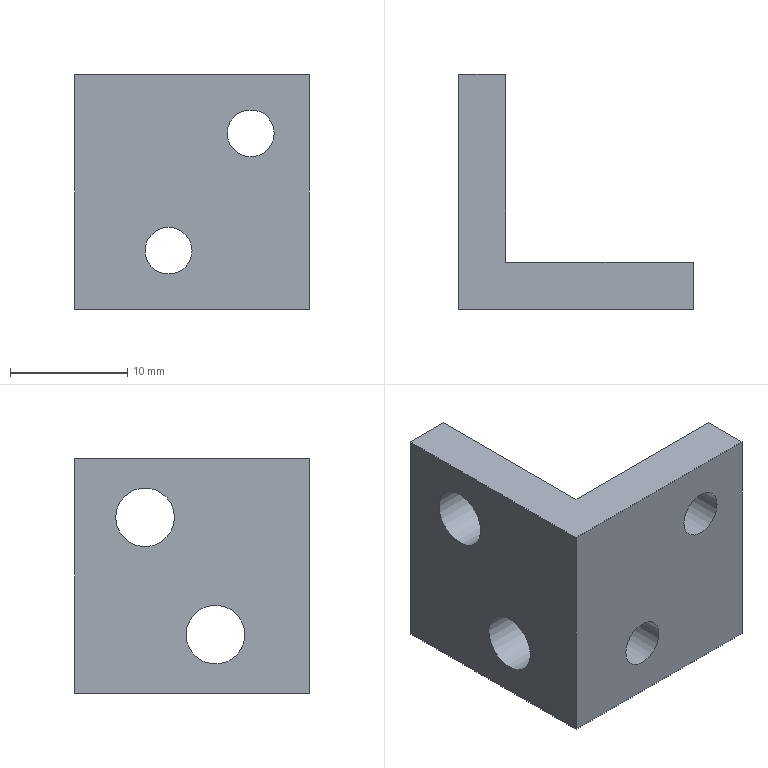Part | STEP file | 1-40.4 | 1 solid | 12 faces | box 20 x 20 x 20 mm | volume 2622 mm3 | plane 8 | cylinder 4 | commonest cylinder face diameters 4 x2 5 x2
STEP:
#1=CARTESIAN_POINT('',(0.,0.,0.));
#2=DIRECTION('',(0.,0.,1.));
#3=DIRECTION('',(1.,0.,0.));
#4=AXIS2_PLACEMENT_3D('',#1,#2,#3);
#5=CARTESIAN_POINT('',(-4.,-10.,-10.));
#6=VERTEX_POINT('',#5);
#7=CARTESIAN_POINT('',(-4.,10.,-10.));
#8=VERTEX_POINT('',#7);
#9=CARTESIAN_POINT('',(-4.,-10.,-10.));
#10=DIRECTION('',(0.,1.,0.));
#11=VECTOR('',#10,1.);
#12=LINE('',#9,#11);
#13=CARTESIAN_POINT('',(-4.,0.,0.));
#14=DIRECTION('',(1.,0.,0.));
#15=DIRECTION('',(0.,1.,0.));
#16=AXIS2_PLACEMENT_3D('',#13,#14,#15);
#17=PLANE('',#16);
#18=CARTESIAN_POINT('',(-10.,-10.));
#19=DIRECTION('',(1.,0.));
#20=VECTOR('',#19,1.);
#21=LINE('',#18,#20);
#22=(GEOMETRIC_REPRESENTATION_CONTEXT(2)PARAMETRIC_REPRESENTATION_CONTEXT()REPRESENTATION_CONTEXT('',''));
#23=DEFINITIONAL_REPRESENTATION('',(#21),#22);
#24=PCURVE('',#17,#23);
#25=CARTESIAN_POINT('',(6.,0.,-10.));
#26=DIRECTION('',(0.,0.,1.));
#27=DIRECTION('',(0.,1.,0.));
#28=AXIS2_PLACEMENT_3D('',#25,#26,#27);
#29=PLANE('',#28);
#30=CARTESIAN_POINT('',(-10.,10.));
#31=DIRECTION('',(1.,0.));
#32=VECTOR('',#31,1.);
#33=LINE('',#30,#32);
#34=(GEOMETRIC_REPRESENTATION_CONTEXT(2)PARAMETRIC_REPRESENTATION_CONTEXT()REPRESENTATION_CONTEXT('',''));
#35=DEFINITIONAL_REPRESENTATION('',(#33),#34);
#36=PCURVE('',#29,#35);
#37=SURFACE_CURVE('',#12,(#24,#36),.PCURVE_S1.);
#38=EDGE_CURVE('',#6,#8,#37,.T.);
#39=ORIENTED_EDGE('',*,*,#38,.T.);
#40=CARTESIAN_POINT('',(-4.,10.,10.));
#41=VERTEX_POINT('',#40);
#42=CARTESIAN_POINT('',(-4.,10.,-10.));
#43=DIRECTION('',(0.,0.,1.));
#44=VECTOR('',#43,1.);
#45=LINE('',#42,#44);
#46=CARTESIAN_POINT('',(10.,-10.));
#47=DIRECTION('',(0.,1.));
#48=VECTOR('',#47,1.);
#49=LINE('',#46,#48);
#50=(GEOMETRIC_REPRESENTATION_CONTEXT(2)PARAMETRIC_REPRESENTATION_CONTEXT()REPRESENTATION_CONTEXT('',''));
#51=DEFINITIONAL_REPRESENTATION('',(#49),#50);
#52=PCURVE('',#17,#51);
#53=CARTESIAN_POINT('',(-2.,10.,0.));
#54=DIRECTION('',(0.,-1.,0.));
#55=DIRECTION('',(0.,0.,1.));
#56=AXIS2_PLACEMENT_3D('',#53,#54,#55);
#57=PLANE('',#56);
#58=CARTESIAN_POINT('',(-10.,2.));
#59=DIRECTION('',(1.,0.));
#60=VECTOR('',#59,1.);
#61=LINE('',#58,#60);
#62=(GEOMETRIC_REPRESENTATION_CONTEXT(2)PARAMETRIC_REPRESENTATION_CONTEXT()REPRESENTATION_CONTEXT('',''));
#63=DEFINITIONAL_REPRESENTATION('',(#61),#62);
#64=PCURVE('',#57,#63);
#65=SURFACE_CURVE('',#45,(#52,#64),.PCURVE_S1.);
#66=EDGE_CURVE('',#8,#41,#65,.T.);
#67=ORIENTED_EDGE('',*,*,#66,.T.);
#68=CARTESIAN_POINT('',(-4.,-10.,10.));
#69=VERTEX_POINT('',#68);
#70=CARTESIAN_POINT('',(-4.,10.,10.));
#71=DIRECTION('',(0.,-1.,0.));
#72=VECTOR('',#71,1.);
#73=LINE('',#70,#72);
#74=CARTESIAN_POINT('',(10.,10.));
#75=DIRECTION('',(-1.,0.));
#76=VECTOR('',#75,1.);
#77=LINE('',#74,#76);
#78=(GEOMETRIC_REPRESENTATION_CONTEXT(2)PARAMETRIC_REPRESENTATION_CONTEXT()REPRESENTATION_CONTEXT('',''));
#79=DEFINITIONAL_REPRESENTATION('',(#77),#78);
#80=PCURVE('',#17,#79);
#81=CARTESIAN_POINT('',(6.,0.,10.));
#82=DIRECTION('',(0.,0.,-1.));
#83=DIRECTION('',(0.,-1.,0.));
#84=AXIS2_PLACEMENT_3D('',#81,#82,#83);
#85=PLANE('',#84);
#86=CARTESIAN_POINT('',(-10.,10.));
#87=DIRECTION('',(1.,0.));
#88=VECTOR('',#87,1.);
#89=LINE('',#86,#88);
#90=(GEOMETRIC_REPRESENTATION_CONTEXT(2)PARAMETRIC_REPRESENTATION_CONTEXT()REPRESENTATION_CONTEXT('',''));
#91=DEFINITIONAL_REPRESENTATION('',(#89),#90);
#92=PCURVE('',#85,#91);
#93=SURFACE_CURVE('',#73,(#80,#92),.PCURVE_S1.);
#94=EDGE_CURVE('',#41,#69,#93,.T.);
#95=ORIENTED_EDGE('',*,*,#94,.T.);
#96=CARTESIAN_POINT('',(-4.,-10.,10.));
#97=DIRECTION('',(0.,0.,-1.));
#98=VECTOR('',#97,1.);
#99=LINE('',#96,#98);
#100=CARTESIAN_POINT('',(-10.,10.));
#101=DIRECTION('',(0.,-1.));
#102=VECTOR('',#101,1.);
#103=LINE('',#100,#102);
#104=(GEOMETRIC_REPRESENTATION_CONTEXT(2)PARAMETRIC_REPRESENTATION_CONTEXT()REPRESENTATION_CONTEXT('',''));
#105=DEFINITIONAL_REPRESENTATION('',(#103),#104);
#106=PCURVE('',#17,#105);
#107=CARTESIAN_POINT('',(8.5,-10.,0.));
#108=DIRECTION('',(0.,1.,0.));
#109=DIRECTION('',(0.,0.,-1.));
#110=AXIS2_PLACEMENT_3D('',#107,#108,#109);
#111=PLANE('',#110);
#112=CARTESIAN_POINT('',(-10.,12.5));
#113=DIRECTION('',(1.,0.));
#114=VECTOR('',#113,1.);
#115=LINE('',#112,#114);
#116=(GEOMETRIC_REPRESENTATION_CONTEXT(2)PARAMETRIC_REPRESENTATION_CONTEXT()REPRESENTATION_CONTEXT('',''));
#117=DEFINITIONAL_REPRESENTATION('',(#115),#116);
#118=PCURVE('',#111,#117);
#119=SURFACE_CURVE('',#99,(#106,#118),.PCURVE_S1.);
#120=EDGE_CURVE('',#69,#6,#119,.T.);
#121=ORIENTED_EDGE('',*,*,#120,.T.);
#122=EDGE_LOOP('',(#39,#67,#95,#121));
#123=FACE_BOUND('',#122,.F.);
#124=CARTESIAN_POINT('',(-4.,0.5,-5.));
#125=VERTEX_POINT('',#124);
#126=CARTESIAN_POINT('',(-4.,-2.,-5.));
#127=DIRECTION('',(-1.,0.,0.));
#128=DIRECTION('',(0.,1.,0.));
#129=AXIS2_PLACEMENT_3D('',#126,#127,#128);
#130=CIRCLE('',#129,2.5);
#131=CARTESIAN_POINT('',(0.5,-5.));
#132=CARTESIAN_POINT('',(0.5,-9.33));
#133=CARTESIAN_POINT('',(-3.25,-7.165));
#134=CARTESIAN_POINT('',(-7.,-5.));
#135=CARTESIAN_POINT('',(-3.25,-2.835));
#136=CARTESIAN_POINT('',(0.5,-0.6699));
#137=CARTESIAN_POINT('',(0.5,-5.));
#138=(BOUNDED_CURVE()B_SPLINE_CURVE(2,(#131,#132,#133,#134,#135,#136,#137),.UNSPECIFIED.,.T.,.F.)B_SPLINE_CURVE_WITH_KNOTS((1,2,2,2,2,1),(-2.094,0.,2.094,4.189,6.283,8.378),.UNSPECIFIED.)CURVE()GEOMETRIC_REPRESENTATION_ITEM()RATIONAL_B_SPLINE_CURVE((1.,0.5,1.,0.5,1.,0.5,1.))REPRESENTATION_ITEM(''));
#139=(GEOMETRIC_REPRESENTATION_CONTEXT(2)PARAMETRIC_REPRESENTATION_CONTEXT()REPRESENTATION_CONTEXT('',''));
#140=DEFINITIONAL_REPRESENTATION('',(#138),#139);
#141=PCURVE('',#17,#140);
#142=CARTESIAN_POINT('',(0.,-2.,-5.));
#143=DIRECTION('',(-1.,0.,0.));
#144=DIRECTION('',(0.,1.,0.));
#145=AXIS2_PLACEMENT_3D('',#142,#143,#144);
#146=CYLINDRICAL_SURFACE('',#145,2.5);
#147=CARTESIAN_POINT('',(0.,4.));
#148=DIRECTION('',(1.,0.));
#149=VECTOR('',#148,1.);
#150=LINE('',#147,#149);
#151=(GEOMETRIC_REPRESENTATION_CONTEXT(2)PARAMETRIC_REPRESENTATION_CONTEXT()REPRESENTATION_CONTEXT('',''));
#152=DEFINITIONAL_REPRESENTATION('',(#150),#151);
#153=PCURVE('',#146,#152);
#154=SURFACE_CURVE('',#130,(#141,#153),.PCURVE_S1.);
#155=EDGE_CURVE('',#125,#125,#154,.T.);
#156=ORIENTED_EDGE('',*,*,#155,.T.);
#157=EDGE_LOOP('',(#156));
#158=FACE_BOUND('',#157,.F.);
#159=CARTESIAN_POINT('',(-4.,6.5,5.));
#160=VERTEX_POINT('',#159);
#161=CARTESIAN_POINT('',(-4.,4.,5.));
#162=DIRECTION('',(-1.,0.,0.));
#163=DIRECTION('',(0.,1.,0.));
#164=AXIS2_PLACEMENT_3D('',#161,#162,#163);
#165=CIRCLE('',#164,2.5);
#166=CARTESIAN_POINT('',(6.5,5.));
#167=CARTESIAN_POINT('',(6.5,0.6699));
#168=CARTESIAN_POINT('',(2.75,2.835));
#169=CARTESIAN_POINT('',(-1.,5.));
#170=CARTESIAN_POINT('',(2.75,7.165));
#171=CARTESIAN_POINT('',(6.5,9.33));
#172=CARTESIAN_POINT('',(6.5,5.));
#173=(BOUNDED_CURVE()B_SPLINE_CURVE(2,(#166,#167,#168,#169,#170,#171,#172),.UNSPECIFIED.,.T.,.F.)B_SPLINE_CURVE_WITH_KNOTS((1,2,2,2,2,1),(-2.094,0.,2.094,4.189,6.283,8.378),.UNSPECIFIED.)CURVE()GEOMETRIC_REPRESENTATION_ITEM()RATIONAL_B_SPLINE_CURVE((1.,0.5,1.,0.5,1.,0.5,1.))REPRESENTATION_ITEM(''));
#174=(GEOMETRIC_REPRESENTATION_CONTEXT(2)PARAMETRIC_REPRESENTATION_CONTEXT()REPRESENTATION_CONTEXT('',''));
#175=DEFINITIONAL_REPRESENTATION('',(#173),#174);
#176=PCURVE('',#17,#175);
#177=CARTESIAN_POINT('',(0.,4.,5.));
#178=DIRECTION('',(-1.,0.,0.));
#179=DIRECTION('',(0.,1.,0.));
#180=AXIS2_PLACEMENT_3D('',#177,#178,#179);
#181=CYLINDRICAL_SURFACE('',#180,2.5);
#182=CARTESIAN_POINT('',(0.,4.));
#183=DIRECTION('',(1.,0.));
#184=VECTOR('',#183,1.);
#185=LINE('',#182,#184);
#186=(GEOMETRIC_REPRESENTATION_CONTEXT(2)PARAMETRIC_REPRESENTATION_CONTEXT()REPRESENTATION_CONTEXT('',''));
#187=DEFINITIONAL_REPRESENTATION('',(#185),#186);
#188=PCURVE('',#181,#187);
#189=SURFACE_CURVE('',#165,(#176,#188),.PCURVE_S1.);
#190=EDGE_CURVE('',#160,#160,#189,.T.);
#191=ORIENTED_EDGE('',*,*,#190,.T.);
#192=EDGE_LOOP('',(#191));
#193=FACE_BOUND('',#192,.F.);
#194=ADVANCED_FACE('',(#123,#158,#193),#17,.F.);
#195=CARTESIAN_POINT('',(0.,-6.,-10.));
#196=VERTEX_POINT('',#195);
#197=CARTESIAN_POINT('',(0.,10.,-10.));
#198=VERTEX_POINT('',#197);
#199=CARTESIAN_POINT('',(0.,-6.,-10.));
#200=DIRECTION('',(0.,1.,0.));
#201=VECTOR('',#200,1.);
#202=LINE('',#199,#201);
#203=CARTESIAN_POINT('',(-6.,6.));
#204=DIRECTION('',(1.,0.));
#205=VECTOR('',#204,1.);
#206=LINE('',#203,#205);
#207=(GEOMETRIC_REPRESENTATION_CONTEXT(2)PARAMETRIC_REPRESENTATION_CONTEXT()REPRESENTATION_CONTEXT('',''));
#208=DEFINITIONAL_REPRESENTATION('',(#206),#207);
#209=PCURVE('',#29,#208);
#210=CARTESIAN_POINT('',(0.,0.,0.));
#211=DIRECTION('',(1.,0.,0.));
#212=DIRECTION('',(0.,1.,0.));
#213=AXIS2_PLACEMENT_3D('',#210,#211,#212);
#214=PLANE('',#213);
#215=CARTESIAN_POINT('',(-6.,-10.));
#216=DIRECTION('',(1.,0.));
#217=VECTOR('',#216,1.);
#218=LINE('',#215,#217);
#219=(GEOMETRIC_REPRESENTATION_CONTEXT(2)PARAMETRIC_REPRESENTATION_CONTEXT()REPRESENTATION_CONTEXT('',''));
#220=DEFINITIONAL_REPRESENTATION('',(#218),#219);
#221=PCURVE('',#214,#220);
#222=SURFACE_CURVE('',#202,(#209,#221),.PCURVE_S1.);
#223=EDGE_CURVE('',#196,#198,#222,.T.);
#224=ORIENTED_EDGE('',*,*,#223,.T.);
#225=CARTESIAN_POINT('',(0.,10.,-10.));
#226=DIRECTION('',(-1.,0.,0.));
#227=VECTOR('',#226,1.);
#228=LINE('',#225,#227);
#229=CARTESIAN_POINT('',(10.,6.));
#230=DIRECTION('',(0.,1.));
#231=VECTOR('',#230,1.);
#232=LINE('',#229,#231);
#233=(GEOMETRIC_REPRESENTATION_CONTEXT(2)PARAMETRIC_REPRESENTATION_CONTEXT()REPRESENTATION_CONTEXT('',''));
#234=DEFINITIONAL_REPRESENTATION('',(#232),#233);
#235=PCURVE('',#29,#234);
#236=CARTESIAN_POINT('',(-10.,-2.));
#237=DIRECTION('',(0.,1.));
#238=VECTOR('',#237,1.);
#239=LINE('',#236,#238);
#240=(GEOMETRIC_REPRESENTATION_CONTEXT(2)PARAMETRIC_REPRESENTATION_CONTEXT()REPRESENTATION_CONTEXT('',''));
#241=DEFINITIONAL_REPRESENTATION('',(#239),#240);
#242=PCURVE('',#57,#241);
#243=SURFACE_CURVE('',#228,(#235,#242),.PCURVE_S1.);
#244=EDGE_CURVE('',#198,#8,#243,.T.);
#245=ORIENTED_EDGE('',*,*,#244,.T.);
#246=ORIENTED_EDGE('',*,*,#38,.F.);
#247=CARTESIAN_POINT('',(16.,-10.,-10.));
#248=VERTEX_POINT('',#247);
#249=CARTESIAN_POINT('',(16.,-10.,-10.));
#250=DIRECTION('',(-1.,0.,0.));
#251=VECTOR('',#250,1.);
#252=LINE('',#249,#251);
#253=CARTESIAN_POINT('',(-10.,-10.));
#254=DIRECTION('',(0.,1.));
#255=VECTOR('',#254,1.);
#256=LINE('',#253,#255);
#257=(GEOMETRIC_REPRESENTATION_CONTEXT(2)PARAMETRIC_REPRESENTATION_CONTEXT()REPRESENTATION_CONTEXT('',''));
#258=DEFINITIONAL_REPRESENTATION('',(#256),#257);
#259=PCURVE('',#29,#258);
#260=CARTESIAN_POINT('',(10.,-7.5));
#261=DIRECTION('',(0.,1.));
#262=VECTOR('',#261,1.);
#263=LINE('',#260,#262);
#264=(GEOMETRIC_REPRESENTATION_CONTEXT(2)PARAMETRIC_REPRESENTATION_CONTEXT()REPRESENTATION_CONTEXT('',''));
#265=DEFINITIONAL_REPRESENTATION('',(#263),#264);
#266=PCURVE('',#111,#265);
#267=SURFACE_CURVE('',#252,(#259,#266),.PCURVE_S1.);
#268=EDGE_CURVE('',#248,#6,#267,.T.);
#269=ORIENTED_EDGE('',*,*,#268,.F.);
#270=CARTESIAN_POINT('',(16.,-6.,-10.));
#271=VERTEX_POINT('',#270);
#272=CARTESIAN_POINT('',(16.,-10.,-10.));
#273=DIRECTION('',(0.,1.,0.));
#274=VECTOR('',#273,1.);
#275=LINE('',#272,#274);
#276=CARTESIAN_POINT('',(-10.,-10.));
#277=DIRECTION('',(1.,0.));
#278=VECTOR('',#277,1.);
#279=LINE('',#276,#278);
#280=(GEOMETRIC_REPRESENTATION_CONTEXT(2)PARAMETRIC_REPRESENTATION_CONTEXT()REPRESENTATION_CONTEXT('',''));
#281=DEFINITIONAL_REPRESENTATION('',(#279),#280);
#282=PCURVE('',#29,#281);
#283=CARTESIAN_POINT('',(16.,-8.,0.));
#284=DIRECTION('',(-1.,0.,0.));
#285=DIRECTION('',(0.,0.,1.));
#286=AXIS2_PLACEMENT_3D('',#283,#284,#285);
#287=PLANE('',#286);
#288=CARTESIAN_POINT('',(-10.,-2.));
#289=DIRECTION('',(0.,1.));
#290=VECTOR('',#289,1.);
#291=LINE('',#288,#290);
#292=(GEOMETRIC_REPRESENTATION_CONTEXT(2)PARAMETRIC_REPRESENTATION_CONTEXT()REPRESENTATION_CONTEXT('',''));
#293=DEFINITIONAL_REPRESENTATION('',(#291),#292);
#294=PCURVE('',#287,#293);
#295=SURFACE_CURVE('',#275,(#282,#294),.PCURVE_S1.);
#296=EDGE_CURVE('',#248,#271,#295,.T.);
#297=ORIENTED_EDGE('',*,*,#296,.T.);
#298=CARTESIAN_POINT('',(0.,-6.,-10.));
#299=DIRECTION('',(1.,0.,0.));
#300=VECTOR('',#299,1.);
#301=LINE('',#298,#300);
#302=CARTESIAN_POINT('',(-6.,6.));
#303=DIRECTION('',(0.,-1.));
#304=VECTOR('',#303,1.);
#305=LINE('',#302,#304);
#306=(GEOMETRIC_REPRESENTATION_CONTEXT(2)PARAMETRIC_REPRESENTATION_CONTEXT()REPRESENTATION_CONTEXT('',''));
#307=DEFINITIONAL_REPRESENTATION('',(#305),#306);
#308=PCURVE('',#29,#307);
#309=CARTESIAN_POINT('',(10.,-6.,0.));
#310=DIRECTION('',(0.,-1.,0.));
#311=DIRECTION('',(1.,0.,0.));
#312=AXIS2_PLACEMENT_3D('',#309,#310,#311);
#313=PLANE('',#312);
#314=CARTESIAN_POINT('',(-10.,-10.));
#315=DIRECTION('',(1.,0.));
#316=VECTOR('',#315,1.);
#317=LINE('',#314,#316);
#318=(GEOMETRIC_REPRESENTATION_CONTEXT(2)PARAMETRIC_REPRESENTATION_CONTEXT()REPRESENTATION_CONTEXT('',''));
#319=DEFINITIONAL_REPRESENTATION('',(#317),#318);
#320=PCURVE('',#313,#319);
#321=SURFACE_CURVE('',#301,(#308,#320),.PCURVE_S1.);
#322=EDGE_CURVE('',#196,#271,#321,.T.);
#323=ORIENTED_EDGE('',*,*,#322,.F.);
#324=EDGE_LOOP('',(#224,#245,#246,#269,#297,#323));
#325=FACE_BOUND('',#324,.F.);
#326=ADVANCED_FACE('',(#325),#29,.F.);
#327=CARTESIAN_POINT('',(0.,10.,10.));
#328=VERTEX_POINT('',#327);
#329=CARTESIAN_POINT('',(0.,10.,-10.));
#330=DIRECTION('',(0.,0.,1.));
#331=VECTOR('',#330,1.);
#332=LINE('',#329,#331);
#333=CARTESIAN_POINT('',(-10.,-2.));
#334=DIRECTION('',(1.,0.));
#335=VECTOR('',#334,1.);
#336=LINE('',#333,#335);
#337=(GEOMETRIC_REPRESENTATION_CONTEXT(2)PARAMETRIC_REPRESENTATION_CONTEXT()REPRESENTATION_CONTEXT('',''));
#338=DEFINITIONAL_REPRESENTATION('',(#336),#337);
#339=PCURVE('',#57,#338);
#340=CARTESIAN_POINT('',(10.,-10.));
#341=DIRECTION('',(0.,1.));
#342=VECTOR('',#341,1.);
#343=LINE('',#340,#342);
#344=(GEOMETRIC_REPRESENTATION_CONTEXT(2)PARAMETRIC_REPRESENTATION_CONTEXT()REPRESENTATION_CONTEXT('',''));
#345=DEFINITIONAL_REPRESENTATION('',(#343),#344);
#346=PCURVE('',#214,#345);
#347=SURFACE_CURVE('',#332,(#339,#346),.PCURVE_S1.);
#348=EDGE_CURVE('',#198,#328,#347,.T.);
#349=ORIENTED_EDGE('',*,*,#348,.T.);
#350=CARTESIAN_POINT('',(0.,10.,10.));
#351=DIRECTION('',(-1.,0.,0.));
#352=VECTOR('',#351,1.);
#353=LINE('',#350,#352);
#354=CARTESIAN_POINT('',(10.,-2.));
#355=DIRECTION('',(0.,1.));
#356=VECTOR('',#355,1.);
#357=LINE('',#354,#356);
#358=(GEOMETRIC_REPRESENTATION_CONTEXT(2)PARAMETRIC_REPRESENTATION_CONTEXT()REPRESENTATION_CONTEXT('',''));
#359=DEFINITIONAL_REPRESENTATION('',(#357),#358);
#360=PCURVE('',#57,#359);
#361=CARTESIAN_POINT('',(-10.,6.));
#362=DIRECTION('',(0.,1.));
#363=VECTOR('',#362,1.);
#364=LINE('',#361,#363);
#365=(GEOMETRIC_REPRESENTATION_CONTEXT(2)PARAMETRIC_REPRESENTATION_CONTEXT()REPRESENTATION_CONTEXT('',''));
#366=DEFINITIONAL_REPRESENTATION('',(#364),#365);
#367=PCURVE('',#85,#366);
#368=SURFACE_CURVE('',#353,(#360,#367),.PCURVE_S1.);
#369=EDGE_CURVE('',#328,#41,#368,.T.);
#370=ORIENTED_EDGE('',*,*,#369,.T.);
#371=ORIENTED_EDGE('',*,*,#66,.F.);
#372=ORIENTED_EDGE('',*,*,#244,.F.);
#373=EDGE_LOOP('',(#349,#370,#371,#372));
#374=FACE_BOUND('',#373,.F.);
#375=ADVANCED_FACE('',(#374),#57,.F.);
#376=ORIENTED_EDGE('',*,*,#94,.F.);
#377=ORIENTED_EDGE('',*,*,#369,.F.);
#378=CARTESIAN_POINT('',(0.,-6.,10.));
#379=VERTEX_POINT('',#378);
#380=CARTESIAN_POINT('',(0.,10.,10.));
#381=DIRECTION('',(0.,-1.,0.));
#382=VECTOR('',#381,1.);
#383=LINE('',#380,#382);
#384=CARTESIAN_POINT('',(-10.,6.));
#385=DIRECTION('',(1.,0.));
#386=VECTOR('',#385,1.);
#387=LINE('',#384,#386);
#388=(GEOMETRIC_REPRESENTATION_CONTEXT(2)PARAMETRIC_REPRESENTATION_CONTEXT()REPRESENTATION_CONTEXT('',''));
#389=DEFINITIONAL_REPRESENTATION('',(#387),#388);
#390=PCURVE('',#85,#389);
#391=CARTESIAN_POINT('',(10.,10.));
#392=DIRECTION('',(-1.,0.));
#393=VECTOR('',#392,1.);
#394=LINE('',#391,#393);
#395=(GEOMETRIC_REPRESENTATION_CONTEXT(2)PARAMETRIC_REPRESENTATION_CONTEXT()REPRESENTATION_CONTEXT('',''));
#396=DEFINITIONAL_REPRESENTATION('',(#394),#395);
#397=PCURVE('',#214,#396);
#398=SURFACE_CURVE('',#383,(#390,#397),.PCURVE_S1.);
#399=EDGE_CURVE('',#328,#379,#398,.T.);
#400=ORIENTED_EDGE('',*,*,#399,.T.);
#401=CARTESIAN_POINT('',(16.,-6.,10.));
#402=VERTEX_POINT('',#401);
#403=CARTESIAN_POINT('',(16.,-6.,10.));
#404=DIRECTION('',(-1.,0.,0.));
#405=VECTOR('',#404,1.);
#406=LINE('',#403,#405);
#407=CARTESIAN_POINT('',(6.,-10.));
#408=DIRECTION('',(0.,1.));
#409=VECTOR('',#408,1.);
#410=LINE('',#407,#409);
#411=(GEOMETRIC_REPRESENTATION_CONTEXT(2)PARAMETRIC_REPRESENTATION_CONTEXT()REPRESENTATION_CONTEXT('',''));
#412=DEFINITIONAL_REPRESENTATION('',(#410),#411);
#413=PCURVE('',#85,#412);
#414=CARTESIAN_POINT('',(6.,10.));
#415=DIRECTION('',(-1.,0.));
#416=VECTOR('',#415,1.);
#417=LINE('',#414,#416);
#418=(GEOMETRIC_REPRESENTATION_CONTEXT(2)PARAMETRIC_REPRESENTATION_CONTEXT()REPRESENTATION_CONTEXT('',''));
#419=DEFINITIONAL_REPRESENTATION('',(#417),#418);
#420=PCURVE('',#313,#419);
#421=SURFACE_CURVE('',#406,(#413,#420),.PCURVE_S1.);
#422=EDGE_CURVE('',#402,#379,#421,.T.);
#423=ORIENTED_EDGE('',*,*,#422,.F.);
#424=CARTESIAN_POINT('',(16.,-10.,10.));
#425=VERTEX_POINT('',#424);
#426=CARTESIAN_POINT('',(16.,-10.,10.));
#427=DIRECTION('',(0.,1.,0.));
#428=VECTOR('',#427,1.);
#429=LINE('',#426,#428);
#430=CARTESIAN_POINT('',(10.,-10.));
#431=DIRECTION('',(-1.,0.));
#432=VECTOR('',#431,1.);
#433=LINE('',#430,#432);
#434=(GEOMETRIC_REPRESENTATION_CONTEXT(2)PARAMETRIC_REPRESENTATION_CONTEXT()REPRESENTATION_CONTEXT('',''));
#435=DEFINITIONAL_REPRESENTATION('',(#433),#434);
#436=PCURVE('',#85,#435);
#437=CARTESIAN_POINT('',(10.,-2.));
#438=DIRECTION('',(0.,1.));
#439=VECTOR('',#438,1.);
#440=LINE('',#437,#439);
#441=(GEOMETRIC_REPRESENTATION_CONTEXT(2)PARAMETRIC_REPRESENTATION_CONTEXT()REPRESENTATION_CONTEXT('',''));
#442=DEFINITIONAL_REPRESENTATION('',(#440),#441);
#443=PCURVE('',#287,#442);
#444=SURFACE_CURVE('',#429,(#436,#443),.PCURVE_S1.);
#445=EDGE_CURVE('',#425,#402,#444,.T.);
#446=ORIENTED_EDGE('',*,*,#445,.F.);
#447=CARTESIAN_POINT('',(-4.,-10.,10.));
#448=DIRECTION('',(1.,0.,0.));
#449=VECTOR('',#448,1.);
#450=LINE('',#447,#449);
#451=CARTESIAN_POINT('',(10.,10.));
#452=DIRECTION('',(0.,-1.));
#453=VECTOR('',#452,1.);
#454=LINE('',#451,#453);
#455=(GEOMETRIC_REPRESENTATION_CONTEXT(2)PARAMETRIC_REPRESENTATION_CONTEXT()REPRESENTATION_CONTEXT('',''));
#456=DEFINITIONAL_REPRESENTATION('',(#454),#455);
#457=PCURVE('',#85,#456);
#458=CARTESIAN_POINT('',(-10.,12.5));
#459=DIRECTION('',(0.,-1.));
#460=VECTOR('',#459,1.);
#461=LINE('',#458,#460);
#462=(GEOMETRIC_REPRESENTATION_CONTEXT(2)PARAMETRIC_REPRESENTATION_CONTEXT()REPRESENTATION_CONTEXT('',''));
#463=DEFINITIONAL_REPRESENTATION('',(#461),#462);
#464=PCURVE('',#111,#463);
#465=SURFACE_CURVE('',#450,(#457,#464),.PCURVE_S1.);
#466=EDGE_CURVE('',#69,#425,#465,.T.);
#467=ORIENTED_EDGE('',*,*,#466,.F.);
#468=EDGE_LOOP('',(#376,#377,#400,#423,#446,#467));
#469=FACE_BOUND('',#468,.F.);
#470=ADVANCED_FACE('',(#469),#85,.F.);
#471=ORIENTED_EDGE('',*,*,#120,.F.);
#472=ORIENTED_EDGE('',*,*,#466,.T.);
#473=CARTESIAN_POINT('',(16.,-10.,-10.));
#474=DIRECTION('',(0.,0.,1.));
#475=VECTOR('',#474,1.);
#476=LINE('',#473,#475);
#477=CARTESIAN_POINT('',(10.,-7.5));
#478=DIRECTION('',(-1.,0.));
#479=VECTOR('',#478,1.);
#480=LINE('',#477,#479);
#481=(GEOMETRIC_REPRESENTATION_CONTEXT(2)PARAMETRIC_REPRESENTATION_CONTEXT()REPRESENTATION_CONTEXT('',''));
#482=DEFINITIONAL_REPRESENTATION('',(#480),#481);
#483=PCURVE('',#111,#482);
#484=CARTESIAN_POINT('',(-10.,-2.));
#485=DIRECTION('',(1.,0.));
#486=VECTOR('',#485,1.);
#487=LINE('',#484,#486);
#488=(GEOMETRIC_REPRESENTATION_CONTEXT(2)PARAMETRIC_REPRESENTATION_CONTEXT()REPRESENTATION_CONTEXT('',''));
#489=DEFINITIONAL_REPRESENTATION('',(#487),#488);
#490=PCURVE('',#287,#489);
#491=SURFACE_CURVE('',#476,(#483,#490),.PCURVE_S1.);
#492=EDGE_CURVE('',#248,#425,#491,.T.);
#493=ORIENTED_EDGE('',*,*,#492,.F.);
#494=ORIENTED_EDGE('',*,*,#268,.T.);
#495=EDGE_LOOP('',(#471,#472,#493,#494));
#496=FACE_BOUND('',#495,.F.);
#497=CARTESIAN_POINT('',(13.,-10.,5.));
#498=VERTEX_POINT('',#497);
#499=CARTESIAN_POINT('',(11.,-10.,5.));
#500=DIRECTION('',(0.,1.,0.));
#501=DIRECTION('',(1.,0.,0.));
#502=AXIS2_PLACEMENT_3D('',#499,#500,#501);
#503=CIRCLE('',#502,2.);
#504=CARTESIAN_POINT('',(-5.,-2.5));
#505=DIRECTION('',(0.,-1.));
#506=AXIS2_PLACEMENT_2D('',#504,#505);
#507=CIRCLE('',#506,2.);
#508=(GEOMETRIC_REPRESENTATION_CONTEXT(2)PARAMETRIC_REPRESENTATION_CONTEXT()REPRESENTATION_CONTEXT('',''));
#509=DEFINITIONAL_REPRESENTATION('',(#507),#508);
#510=PCURVE('',#111,#509);
#511=CARTESIAN_POINT('',(11.,-10.,5.));
#512=DIRECTION('',(0.,1.,0.));
#513=DIRECTION('',(1.,0.,0.));
#514=AXIS2_PLACEMENT_3D('',#511,#512,#513);
#515=CYLINDRICAL_SURFACE('',#514,2.);
#516=CARTESIAN_POINT('',(0.,0.));
#517=DIRECTION('',(1.,0.));
#518=VECTOR('',#517,1.);
#519=LINE('',#516,#518);
#520=(GEOMETRIC_REPRESENTATION_CONTEXT(2)PARAMETRIC_REPRESENTATION_CONTEXT()REPRESENTATION_CONTEXT('',''));
#521=DEFINITIONAL_REPRESENTATION('',(#519),#520);
#522=PCURVE('',#515,#521);
#523=SURFACE_CURVE('',#503,(#510,#522),.PCURVE_S1.);
#524=EDGE_CURVE('',#498,#498,#523,.T.);
#525=ORIENTED_EDGE('',*,*,#524,.F.);
#526=EDGE_LOOP('',(#525));
#527=FACE_BOUND('',#526,.F.);
#528=CARTESIAN_POINT('',(6.,-10.,-5.));
#529=VERTEX_POINT('',#528);
#530=CARTESIAN_POINT('',(4.,-10.,-5.));
#531=DIRECTION('',(0.,1.,0.));
#532=DIRECTION('',(1.,0.,0.));
#533=AXIS2_PLACEMENT_3D('',#530,#531,#532);
#534=CIRCLE('',#533,2.);
#535=CARTESIAN_POINT('',(5.,4.5));
#536=DIRECTION('',(0.,-1.));
#537=AXIS2_PLACEMENT_2D('',#535,#536);
#538=CIRCLE('',#537,2.);
#539=(GEOMETRIC_REPRESENTATION_CONTEXT(2)PARAMETRIC_REPRESENTATION_CONTEXT()REPRESENTATION_CONTEXT('',''));
#540=DEFINITIONAL_REPRESENTATION('',(#538),#539);
#541=PCURVE('',#111,#540);
#542=CARTESIAN_POINT('',(4.,-10.,-5.));
#543=DIRECTION('',(0.,1.,0.));
#544=DIRECTION('',(1.,0.,0.));
#545=AXIS2_PLACEMENT_3D('',#542,#543,#544);
#546=CYLINDRICAL_SURFACE('',#545,2.);
#547=CARTESIAN_POINT('',(0.,0.));
#548=DIRECTION('',(1.,0.));
#549=VECTOR('',#548,1.);
#550=LINE('',#547,#549);
#551=(GEOMETRIC_REPRESENTATION_CONTEXT(2)PARAMETRIC_REPRESENTATION_CONTEXT()REPRESENTATION_CONTEXT('',''));
#552=DEFINITIONAL_REPRESENTATION('',(#550),#551);
#553=PCURVE('',#546,#552);
#554=SURFACE_CURVE('',#534,(#541,#553),.PCURVE_S1.);
#555=EDGE_CURVE('',#529,#529,#554,.T.);
#556=ORIENTED_EDGE('',*,*,#555,.F.);
#557=EDGE_LOOP('',(#556));
#558=FACE_BOUND('',#557,.F.);
#559=ADVANCED_FACE('',(#496,#527,#558),#111,.F.);
#560=CARTESIAN_POINT('',(0.,0.5,-5.));
#561=VERTEX_POINT('',#560);
#562=CARTESIAN_POINT('',(0.,-2.,-5.));
#563=DIRECTION('',(-1.,0.,0.));
#564=DIRECTION('',(0.,1.,0.));
#565=AXIS2_PLACEMENT_3D('',#562,#563,#564);
#566=CIRCLE('',#565,2.5);
#567=CARTESIAN_POINT('',(0.,0.));
#568=DIRECTION('',(1.,0.));
#569=VECTOR('',#568,1.);
#570=LINE('',#567,#569);
#571=(GEOMETRIC_REPRESENTATION_CONTEXT(2)PARAMETRIC_REPRESENTATION_CONTEXT()REPRESENTATION_CONTEXT('',''));
#572=DEFINITIONAL_REPRESENTATION('',(#570),#571);
#573=PCURVE('',#146,#572);
#574=CARTESIAN_POINT('',(0.5,-5.));
#575=CARTESIAN_POINT('',(0.5,-9.33));
#576=CARTESIAN_POINT('',(-3.25,-7.165));
#577=CARTESIAN_POINT('',(-7.,-5.));
#578=CARTESIAN_POINT('',(-3.25,-2.835));
#579=CARTESIAN_POINT('',(0.5,-0.6699));
#580=CARTESIAN_POINT('',(0.5,-5.));
#581=(BOUNDED_CURVE()B_SPLINE_CURVE(2,(#574,#575,#576,#577,#578,#579,#580),.UNSPECIFIED.,.T.,.F.)B_SPLINE_CURVE_WITH_KNOTS((1,2,2,2,2,1),(-2.094,0.,2.094,4.189,6.283,8.378),.UNSPECIFIED.)CURVE()GEOMETRIC_REPRESENTATION_ITEM()RATIONAL_B_SPLINE_CURVE((1.,0.5,1.,0.5,1.,0.5,1.))REPRESENTATION_ITEM(''));
#582=(GEOMETRIC_REPRESENTATION_CONTEXT(2)PARAMETRIC_REPRESENTATION_CONTEXT()REPRESENTATION_CONTEXT('',''));
#583=DEFINITIONAL_REPRESENTATION('',(#581),#582);
#584=PCURVE('',#214,#583);
#585=SURFACE_CURVE('',#566,(#573,#584),.PCURVE_S1.);
#586=EDGE_CURVE('',#561,#561,#585,.T.);
#587=ORIENTED_EDGE('',*,*,#586,.T.);
#588=CARTESIAN_POINT('',(0.,0.5,-5.));
#589=DIRECTION('',(-1.,0.,0.));
#590=VECTOR('',#589,1.);
#591=LINE('',#588,#590);
#592=CARTESIAN_POINT('',(6.283,0.));
#593=DIRECTION('',(0.,1.));
#594=VECTOR('',#593,1.);
#595=LINE('',#592,#594);
#596=(GEOMETRIC_REPRESENTATION_CONTEXT(2)PARAMETRIC_REPRESENTATION_CONTEXT()REPRESENTATION_CONTEXT('',''));
#597=DEFINITIONAL_REPRESENTATION('',(#595),#596);
#598=PCURVE('',#146,#597);
#599=CARTESIAN_POINT('',(0.,0.));
#600=DIRECTION('',(0.,1.));
#601=VECTOR('',#600,1.);
#602=LINE('',#599,#601);
#603=(GEOMETRIC_REPRESENTATION_CONTEXT(2)PARAMETRIC_REPRESENTATION_CONTEXT()REPRESENTATION_CONTEXT('',''));
#604=DEFINITIONAL_REPRESENTATION('',(#602),#603);
#605=PCURVE('',#146,#604);
#606=SEAM_CURVE('',#591,(#598,#605),.PCURVE_S1.);
#607=EDGE_CURVE('',#561,#125,#606,.T.);
#608=ORIENTED_EDGE('',*,*,#607,.T.);
#609=ORIENTED_EDGE('',*,*,#155,.F.);
#610=ORIENTED_EDGE('',*,*,#607,.F.);
#611=EDGE_LOOP('',(#587,#608,#609,#610));
#612=FACE_BOUND('',#611,.F.);
#613=ADVANCED_FACE('',(#612),#146,.F.);
#614=CARTESIAN_POINT('',(0.,6.5,5.));
#615=VERTEX_POINT('',#614);
#616=CARTESIAN_POINT('',(0.,4.,5.));
#617=DIRECTION('',(-1.,0.,0.));
#618=DIRECTION('',(0.,1.,0.));
#619=AXIS2_PLACEMENT_3D('',#616,#617,#618);
#620=CIRCLE('',#619,2.5);
#621=CARTESIAN_POINT('',(0.,0.));
#622=DIRECTION('',(1.,0.));
#623=VECTOR('',#622,1.);
#624=LINE('',#621,#623);
#625=(GEOMETRIC_REPRESENTATION_CONTEXT(2)PARAMETRIC_REPRESENTATION_CONTEXT()REPRESENTATION_CONTEXT('',''));
#626=DEFINITIONAL_REPRESENTATION('',(#624),#625);
#627=PCURVE('',#181,#626);
#628=CARTESIAN_POINT('',(6.5,5.));
#629=CARTESIAN_POINT('',(6.5,0.6699));
#630=CARTESIAN_POINT('',(2.75,2.835));
#631=CARTESIAN_POINT('',(-1.,5.));
#632=CARTESIAN_POINT('',(2.75,7.165));
#633=CARTESIAN_POINT('',(6.5,9.33));
#634=CARTESIAN_POINT('',(6.5,5.));
#635=(BOUNDED_CURVE()B_SPLINE_CURVE(2,(#628,#629,#630,#631,#632,#633,#634),.UNSPECIFIED.,.T.,.F.)B_SPLINE_CURVE_WITH_KNOTS((1,2,2,2,2,1),(-2.094,0.,2.094,4.189,6.283,8.378),.UNSPECIFIED.)CURVE()GEOMETRIC_REPRESENTATION_ITEM()RATIONAL_B_SPLINE_CURVE((1.,0.5,1.,0.5,1.,0.5,1.))REPRESENTATION_ITEM(''));
#636=(GEOMETRIC_REPRESENTATION_CONTEXT(2)PARAMETRIC_REPRESENTATION_CONTEXT()REPRESENTATION_CONTEXT('',''));
#637=DEFINITIONAL_REPRESENTATION('',(#635),#636);
#638=PCURVE('',#214,#637);
#639=SURFACE_CURVE('',#620,(#627,#638),.PCURVE_S1.);
#640=EDGE_CURVE('',#615,#615,#639,.T.);
#641=ORIENTED_EDGE('',*,*,#640,.T.);
#642=CARTESIAN_POINT('',(0.,6.5,5.));
#643=DIRECTION('',(-1.,0.,0.));
#644=VECTOR('',#643,1.);
#645=LINE('',#642,#644);
#646=CARTESIAN_POINT('',(6.283,0.));
#647=DIRECTION('',(0.,1.));
#648=VECTOR('',#647,1.);
#649=LINE('',#646,#648);
#650=(GEOMETRIC_REPRESENTATION_CONTEXT(2)PARAMETRIC_REPRESENTATION_CONTEXT()REPRESENTATION_CONTEXT('',''));
#651=DEFINITIONAL_REPRESENTATION('',(#649),#650);
#652=PCURVE('',#181,#651);
#653=CARTESIAN_POINT('',(0.,0.));
#654=DIRECTION('',(0.,1.));
#655=VECTOR('',#654,1.);
#656=LINE('',#653,#655);
#657=(GEOMETRIC_REPRESENTATION_CONTEXT(2)PARAMETRIC_REPRESENTATION_CONTEXT()REPRESENTATION_CONTEXT('',''));
#658=DEFINITIONAL_REPRESENTATION('',(#656),#657);
#659=PCURVE('',#181,#658);
#660=SEAM_CURVE('',#645,(#652,#659),.PCURVE_S1.);
#661=EDGE_CURVE('',#615,#160,#660,.T.);
#662=ORIENTED_EDGE('',*,*,#661,.T.);
#663=ORIENTED_EDGE('',*,*,#190,.F.);
#664=ORIENTED_EDGE('',*,*,#661,.F.);
#665=EDGE_LOOP('',(#641,#662,#663,#664));
#666=FACE_BOUND('',#665,.F.);
#667=ADVANCED_FACE('',(#666),#181,.F.);
#668=ORIENTED_EDGE('',*,*,#348,.T.);
#669=ORIENTED_EDGE('',*,*,#399,.T.);
#670=CARTESIAN_POINT('',(0.,-6.,10.));
#671=DIRECTION('',(0.,0.,-1.));
#672=VECTOR('',#671,1.);
#673=LINE('',#670,#672);
#674=CARTESIAN_POINT('',(-6.,10.));
#675=DIRECTION('',(0.,-1.));
#676=VECTOR('',#675,1.);
#677=LINE('',#674,#676);
#678=(GEOMETRIC_REPRESENTATION_CONTEXT(2)PARAMETRIC_REPRESENTATION_CONTEXT()REPRESENTATION_CONTEXT('',''));
#679=DEFINITIONAL_REPRESENTATION('',(#677),#678);
#680=PCURVE('',#214,#679);
#681=CARTESIAN_POINT('',(-10.,10.));
#682=DIRECTION('',(0.,-1.));
#683=VECTOR('',#682,1.);
#684=LINE('',#681,#683);
#685=(GEOMETRIC_REPRESENTATION_CONTEXT(2)PARAMETRIC_REPRESENTATION_CONTEXT()REPRESENTATION_CONTEXT('',''));
#686=DEFINITIONAL_REPRESENTATION('',(#684),#685);
#687=PCURVE('',#313,#686);
#688=SURFACE_CURVE('',#673,(#680,#687),.PCURVE_S1.);
#689=EDGE_CURVE('',#379,#196,#688,.T.);
#690=ORIENTED_EDGE('',*,*,#689,.T.);
#691=ORIENTED_EDGE('',*,*,#223,.T.);
#692=EDGE_LOOP('',(#668,#669,#690,#691));
#693=FACE_BOUND('',#692,.T.);
#694=ORIENTED_EDGE('',*,*,#586,.T.);
#695=EDGE_LOOP('',(#694));
#696=FACE_BOUND('',#695,.T.);
#697=ORIENTED_EDGE('',*,*,#640,.T.);
#698=EDGE_LOOP('',(#697));
#699=FACE_BOUND('',#698,.T.);
#700=ADVANCED_FACE('',(#693,#696,#699),#214,.T.);
#701=CARTESIAN_POINT('',(16.,-6.,-10.));
#702=DIRECTION('',(0.,0.,1.));
#703=VECTOR('',#702,1.);
#704=LINE('',#701,#703);
#705=CARTESIAN_POINT('',(6.,-10.));
#706=DIRECTION('',(0.,1.));
#707=VECTOR('',#706,1.);
#708=LINE('',#705,#707);
#709=(GEOMETRIC_REPRESENTATION_CONTEXT(2)PARAMETRIC_REPRESENTATION_CONTEXT()REPRESENTATION_CONTEXT('',''));
#710=DEFINITIONAL_REPRESENTATION('',(#708),#709);
#711=PCURVE('',#313,#710);
#712=CARTESIAN_POINT('',(-10.,2.));
#713=DIRECTION('',(1.,0.));
#714=VECTOR('',#713,1.);
#715=LINE('',#712,#714);
#716=(GEOMETRIC_REPRESENTATION_CONTEXT(2)PARAMETRIC_REPRESENTATION_CONTEXT()REPRESENTATION_CONTEXT('',''));
#717=DEFINITIONAL_REPRESENTATION('',(#715),#716);
#718=PCURVE('',#287,#717);
#719=SURFACE_CURVE('',#704,(#711,#718),.PCURVE_S1.);
#720=EDGE_CURVE('',#271,#402,#719,.T.);
#721=ORIENTED_EDGE('',*,*,#720,.T.);
#722=ORIENTED_EDGE('',*,*,#422,.T.);
#723=ORIENTED_EDGE('',*,*,#689,.T.);
#724=ORIENTED_EDGE('',*,*,#322,.T.);
#725=EDGE_LOOP('',(#721,#722,#723,#724));
#726=FACE_BOUND('',#725,.F.);
#727=CARTESIAN_POINT('',(6.,-6.,-5.));
#728=VERTEX_POINT('',#727);
#729=CARTESIAN_POINT('',(4.,-6.,-5.));
#730=DIRECTION('',(0.,1.,0.));
#731=DIRECTION('',(1.,0.,0.));
#732=AXIS2_PLACEMENT_3D('',#729,#730,#731);
#733=CIRCLE('',#732,2.);
#734=CARTESIAN_POINT('',(-4.,-5.));
#735=CARTESIAN_POINT('',(-4.,-8.464));
#736=CARTESIAN_POINT('',(-7.,-6.732));
#737=CARTESIAN_POINT('',(-10.,-5.));
#738=CARTESIAN_POINT('',(-7.,-3.268));
#739=CARTESIAN_POINT('',(-4.,-1.536));
#740=CARTESIAN_POINT('',(-4.,-5.));
#741=(BOUNDED_CURVE()B_SPLINE_CURVE(2,(#734,#735,#736,#737,#738,#739,#740),.UNSPECIFIED.,.T.,.F.)B_SPLINE_CURVE_WITH_KNOTS((1,2,2,2,2,1),(-2.094,0.,2.094,4.189,6.283,8.378),.UNSPECIFIED.)CURVE()GEOMETRIC_REPRESENTATION_ITEM()RATIONAL_B_SPLINE_CURVE((1.,0.5,1.,0.5,1.,0.5,1.))REPRESENTATION_ITEM(''));
#742=(GEOMETRIC_REPRESENTATION_CONTEXT(2)PARAMETRIC_REPRESENTATION_CONTEXT()REPRESENTATION_CONTEXT('',''));
#743=DEFINITIONAL_REPRESENTATION('',(#741),#742);
#744=PCURVE('',#313,#743);
#745=CARTESIAN_POINT('',(0.,4.));
#746=DIRECTION('',(1.,0.));
#747=VECTOR('',#746,1.);
#748=LINE('',#745,#747);
#749=(GEOMETRIC_REPRESENTATION_CONTEXT(2)PARAMETRIC_REPRESENTATION_CONTEXT()REPRESENTATION_CONTEXT('',''));
#750=DEFINITIONAL_REPRESENTATION('',(#748),#749);
#751=PCURVE('',#546,#750);
#752=SURFACE_CURVE('',#733,(#744,#751),.PCURVE_S1.);
#753=EDGE_CURVE('',#728,#728,#752,.T.);
#754=ORIENTED_EDGE('',*,*,#753,.T.);
#755=EDGE_LOOP('',(#754));
#756=FACE_BOUND('',#755,.F.);
#757=CARTESIAN_POINT('',(13.,-6.,5.));
#758=VERTEX_POINT('',#757);
#759=CARTESIAN_POINT('',(11.,-6.,5.));
#760=DIRECTION('',(0.,1.,0.));
#761=DIRECTION('',(1.,0.,0.));
#762=AXIS2_PLACEMENT_3D('',#759,#760,#761);
#763=CIRCLE('',#762,2.);
#764=CARTESIAN_POINT('',(3.,5.));
#765=CARTESIAN_POINT('',(3.,1.536));
#766=CARTESIAN_POINT('',(0.,3.268));
#767=CARTESIAN_POINT('',(-3.,5.));
#768=CARTESIAN_POINT('',(0.,6.732));
#769=CARTESIAN_POINT('',(3.,8.464));
#770=CARTESIAN_POINT('',(3.,5.));
#771=(BOUNDED_CURVE()B_SPLINE_CURVE(2,(#764,#765,#766,#767,#768,#769,#770),.UNSPECIFIED.,.T.,.F.)B_SPLINE_CURVE_WITH_KNOTS((1,2,2,2,2,1),(-2.094,0.,2.094,4.189,6.283,8.378),.UNSPECIFIED.)CURVE()GEOMETRIC_REPRESENTATION_ITEM()RATIONAL_B_SPLINE_CURVE((1.,0.5,1.,0.5,1.,0.5,1.))REPRESENTATION_ITEM(''));
#772=(GEOMETRIC_REPRESENTATION_CONTEXT(2)PARAMETRIC_REPRESENTATION_CONTEXT()REPRESENTATION_CONTEXT('',''));
#773=DEFINITIONAL_REPRESENTATION('',(#771),#772);
#774=PCURVE('',#313,#773);
#775=CARTESIAN_POINT('',(0.,4.));
#776=DIRECTION('',(1.,0.));
#777=VECTOR('',#776,1.);
#778=LINE('',#775,#777);
#779=(GEOMETRIC_REPRESENTATION_CONTEXT(2)PARAMETRIC_REPRESENTATION_CONTEXT()REPRESENTATION_CONTEXT('',''));
#780=DEFINITIONAL_REPRESENTATION('',(#778),#779);
#781=PCURVE('',#515,#780);
#782=SURFACE_CURVE('',#763,(#774,#781),.PCURVE_S1.);
#783=EDGE_CURVE('',#758,#758,#782,.T.);
#784=ORIENTED_EDGE('',*,*,#783,.T.);
#785=EDGE_LOOP('',(#784));
#786=FACE_BOUND('',#785,.F.);
#787=ADVANCED_FACE('',(#726,#756,#786),#313,.F.);
#788=ORIENTED_EDGE('',*,*,#492,.T.);
#789=ORIENTED_EDGE('',*,*,#445,.T.);
#790=ORIENTED_EDGE('',*,*,#720,.F.);
#791=ORIENTED_EDGE('',*,*,#296,.F.);
#792=EDGE_LOOP('',(#788,#789,#790,#791));
#793=FACE_BOUND('',#792,.F.);
#794=ADVANCED_FACE('',(#793),#287,.F.);
#795=ORIENTED_EDGE('',*,*,#555,.T.);
#796=CARTESIAN_POINT('',(6.,-10.,-5.));
#797=DIRECTION('',(0.,1.,0.));
#798=VECTOR('',#797,1.);
#799=LINE('',#796,#798);
#800=CARTESIAN_POINT('',(6.283,0.));
#801=DIRECTION('',(0.,1.));
#802=VECTOR('',#801,1.);
#803=LINE('',#800,#802);
#804=(GEOMETRIC_REPRESENTATION_CONTEXT(2)PARAMETRIC_REPRESENTATION_CONTEXT()REPRESENTATION_CONTEXT('',''));
#805=DEFINITIONAL_REPRESENTATION('',(#803),#804);
#806=PCURVE('',#546,#805);
#807=CARTESIAN_POINT('',(0.,0.));
#808=DIRECTION('',(0.,1.));
#809=VECTOR('',#808,1.);
#810=LINE('',#807,#809);
#811=(GEOMETRIC_REPRESENTATION_CONTEXT(2)PARAMETRIC_REPRESENTATION_CONTEXT()REPRESENTATION_CONTEXT('',''));
#812=DEFINITIONAL_REPRESENTATION('',(#810),#811);
#813=PCURVE('',#546,#812);
#814=SEAM_CURVE('',#799,(#806,#813),.PCURVE_S1.);
#815=EDGE_CURVE('',#529,#728,#814,.T.);
#816=ORIENTED_EDGE('',*,*,#815,.T.);
#817=ORIENTED_EDGE('',*,*,#753,.F.);
#818=ORIENTED_EDGE('',*,*,#815,.F.);
#819=EDGE_LOOP('',(#795,#816,#817,#818));
#820=FACE_BOUND('',#819,.F.);
#821=ADVANCED_FACE('',(#820),#546,.F.);
#822=ORIENTED_EDGE('',*,*,#524,.T.);
#823=CARTESIAN_POINT('',(13.,-10.,5.));
#824=DIRECTION('',(0.,1.,0.));
#825=VECTOR('',#824,1.);
#826=LINE('',#823,#825);
#827=CARTESIAN_POINT('',(6.283,0.));
#828=DIRECTION('',(0.,1.));
#829=VECTOR('',#828,1.);
#830=LINE('',#827,#829);
#831=(GEOMETRIC_REPRESENTATION_CONTEXT(2)PARAMETRIC_REPRESENTATION_CONTEXT()REPRESENTATION_CONTEXT('',''));
#832=DEFINITIONAL_REPRESENTATION('',(#830),#831);
#833=PCURVE('',#515,#832);
#834=CARTESIAN_POINT('',(0.,0.));
#835=DIRECTION('',(0.,1.));
#836=VECTOR('',#835,1.);
#837=LINE('',#834,#836);
#838=(GEOMETRIC_REPRESENTATION_CONTEXT(2)PARAMETRIC_REPRESENTATION_CONTEXT()REPRESENTATION_CONTEXT('',''));
#839=DEFINITIONAL_REPRESENTATION('',(#837),#838);
#840=PCURVE('',#515,#839);
#841=SEAM_CURVE('',#826,(#833,#840),.PCURVE_S1.);
#842=EDGE_CURVE('',#498,#758,#841,.T.);
#843=ORIENTED_EDGE('',*,*,#842,.T.);
#844=ORIENTED_EDGE('',*,*,#783,.F.);
#845=ORIENTED_EDGE('',*,*,#842,.F.);
#846=EDGE_LOOP('',(#822,#843,#844,#845));
#847=FACE_BOUND('',#846,.F.);
#848=ADVANCED_FACE('',(#847),#515,.F.);
#849=CLOSED_SHELL('',(#194,#326,#375,#470,#559,#613,#667,#700,#787,#794,#821,#848));
#850=MANIFOLD_SOLID_BREP('',#849);
#851=(LENGTH_UNIT()NAMED_UNIT(*)SI_UNIT(.MILLI.,.METRE.));
#852=UNCERTAINTY_MEASURE_WITH_UNIT(LENGTH_MEASURE(0.0000001),#851,'','');
#853=(NAMED_UNIT(*)PLANE_ANGLE_UNIT()SI_UNIT($,.RADIAN.));
#854=(NAMED_UNIT(*)SI_UNIT($,.STERADIAN.)SOLID_ANGLE_UNIT());
#855=(GEOMETRIC_REPRESENTATION_CONTEXT(3)GLOBAL_UNCERTAINTY_ASSIGNED_CONTEXT((#852))GLOBAL_UNIT_ASSIGNED_CONTEXT((#851,#853,#854))REPRESENTATION_CONTEXT('',''));
#856=ADVANCED_BREP_SHAPE_REPRESENTATION('',(#4,#850),#855);